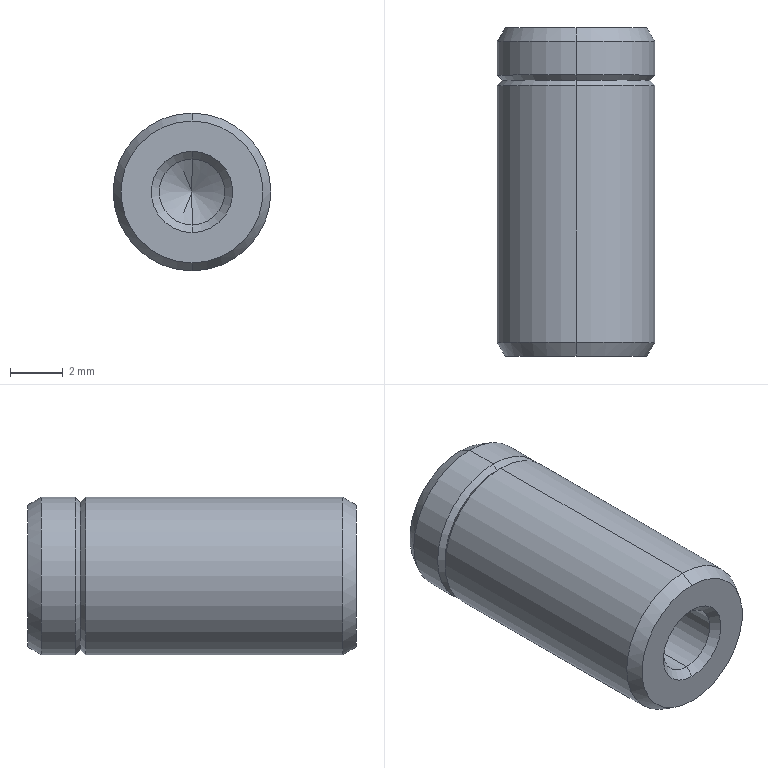Part | STEP file | MOP-12.5-1.step-2.STEP.STEP-60.STEP | 1 solid | 26 faces | box 6 x 12.5 x 6 mm | volume 302.452 mm3 | cone 16 | cylinder 8 | plane 2 | commonest cylinder face diameters 2.5 x4 6 x4
STEP:
#1=CARTESIAN_POINT('',(0.,10.3,3.));
#2=VERTEX_POINT('',#1);
#3=CARTESIAN_POINT('',(0.,10.3,-3.));
#4=VERTEX_POINT('',#3);
#5=CARTESIAN_POINT('',(0.,10.3,0.));
#6=DIRECTION('',(0.,1.,0.));
#7=DIRECTION('',(0.,0.,-1.));
#8=AXIS2_PLACEMENT_3D('',#5,#6,#7);
#9=CIRCLE('',#8,3.);
#10=EDGE_CURVE('',#2,#4,#9,.T.);
#11=ORIENTED_EDGE('',*,*,#10,.F.);
#12=CARTESIAN_POINT('',(0.,0.5196,3.));
#13=VERTEX_POINT('',#12);
#14=CARTESIAN_POINT('',(0.,12.5,3.));
#15=DIRECTION('',(0.,-1.,0.));
#16=VECTOR('',#15,1000.);
#17=LINE('',#14,#16);
#18=EDGE_CURVE('',#2,#13,#17,.T.);
#19=ORIENTED_EDGE('',*,*,#18,.T.);
#20=CARTESIAN_POINT('',(0.,0.5196,-3.));
#21=VERTEX_POINT('',#20);
#22=CARTESIAN_POINT('',(0.,0.5196,0.));
#23=DIRECTION('',(0.,1.,0.));
#24=DIRECTION('',(0.,0.,1.));
#25=AXIS2_PLACEMENT_3D('',#22,#23,#24);
#26=CIRCLE('',#25,3.);
#27=EDGE_CURVE('',#13,#21,#26,.T.);
#28=ORIENTED_EDGE('',*,*,#27,.T.);
#29=CARTESIAN_POINT('',(0.,12.5,-3.));
#30=DIRECTION('',(0.,-1.,0.));
#31=VECTOR('',#30,1000.);
#32=LINE('',#29,#31);
#33=EDGE_CURVE('',#4,#21,#32,.T.);
#34=ORIENTED_EDGE('',*,*,#33,.F.);
#35=EDGE_LOOP('',(#11,#19,#28,#34));
#36=FACE_OUTER_BOUND('',#35,.T.);
#37=CARTESIAN_POINT('',(0.,12.5,0.));
#38=DIRECTION('',(0.,-1.,0.));
#39=DIRECTION('',(0.,0.,-1.));
#40=AXIS2_PLACEMENT_3D('',#37,#38,#39);
#41=CYLINDRICAL_SURFACE('',#40,3.);
#42=ADVANCED_FACE('',(#36),#41,.T.);
#43=CARTESIAN_POINT('',(0.,0.,-2.7));
#44=VERTEX_POINT('',#43);
#45=CARTESIAN_POINT('',(0.,0.,2.7));
#46=VERTEX_POINT('',#45);
#47=CARTESIAN_POINT('',(0.,0.,0.));
#48=DIRECTION('',(0.,-1.,0.));
#49=DIRECTION('',(0.,0.,1.));
#50=AXIS2_PLACEMENT_3D('',#47,#48,#49);
#51=CIRCLE('',#50,2.7);
#52=EDGE_CURVE('',#44,#46,#51,.T.);
#53=ORIENTED_EDGE('',*,*,#52,.F.);
#54=CARTESIAN_POINT('',(0.,0.5196,-3.));
#55=DIRECTION('',(0.,0.866,-0.5));
#56=VECTOR('',#55,1000.);
#57=LINE('',#54,#56);
#58=EDGE_CURVE('',#44,#21,#57,.T.);
#59=ORIENTED_EDGE('',*,*,#58,.T.);
#60=ORIENTED_EDGE('',*,*,#27,.F.);
#61=CARTESIAN_POINT('',(0.,0.5196,3.));
#62=DIRECTION('',(0.,0.866,0.5));
#63=VECTOR('',#62,1000.);
#64=LINE('',#61,#63);
#65=EDGE_CURVE('',#46,#13,#64,.T.);
#66=ORIENTED_EDGE('',*,*,#65,.F.);
#67=EDGE_LOOP('',(#53,#59,#60,#66));
#68=FACE_OUTER_BOUND('',#67,.T.);
#69=CARTESIAN_POINT('',(0.,0.5196,0.));
#70=DIRECTION('',(0.,1.,0.));
#71=DIRECTION('',(0.,0.,1.));
#72=AXIS2_PLACEMENT_3D('',#69,#70,#71);
#73=CONICAL_SURFACE('',#72,3.,0.5236);
#74=ADVANCED_FACE('',(#68),#73,.T.);
#75=CARTESIAN_POINT('',(0.,0.3,1.25));
#76=VERTEX_POINT('',#75);
#77=CARTESIAN_POINT('',(0.,0.3,-1.25));
#78=VERTEX_POINT('',#77);
#79=CARTESIAN_POINT('',(0.,0.3,0.));
#80=DIRECTION('',(0.,-1.,0.));
#81=DIRECTION('',(0.,0.,1.));
#82=AXIS2_PLACEMENT_3D('',#79,#80,#81);
#83=CIRCLE('',#82,1.25);
#84=EDGE_CURVE('',#76,#78,#83,.T.);
#85=ORIENTED_EDGE('',*,*,#84,.F.);
#86=CARTESIAN_POINT('',(0.,0.,1.55));
#87=VERTEX_POINT('',#86);
#88=CARTESIAN_POINT('',(0.,0.3,1.25));
#89=DIRECTION('',(0.,-0.7071,0.7071));
#90=VECTOR('',#89,1000.);
#91=LINE('',#88,#90);
#92=EDGE_CURVE('',#76,#87,#91,.T.);
#93=ORIENTED_EDGE('',*,*,#92,.T.);
#94=CARTESIAN_POINT('',(0.,0.,-1.55));
#95=VERTEX_POINT('',#94);
#96=CARTESIAN_POINT('',(0.,0.,0.));
#97=DIRECTION('',(0.,1.,0.));
#98=DIRECTION('',(0.,0.,1.));
#99=AXIS2_PLACEMENT_3D('',#96,#97,#98);
#100=CIRCLE('',#99,1.55);
#101=EDGE_CURVE('',#95,#87,#100,.T.);
#102=ORIENTED_EDGE('',*,*,#101,.F.);
#103=CARTESIAN_POINT('',(0.,0.3,-1.25));
#104=DIRECTION('',(0.,-0.7071,-0.7071));
#105=VECTOR('',#104,1000.);
#106=LINE('',#103,#105);
#107=EDGE_CURVE('',#78,#95,#106,.T.);
#108=ORIENTED_EDGE('',*,*,#107,.F.);
#109=EDGE_LOOP('',(#85,#93,#102,#108));
#110=FACE_OUTER_BOUND('',#109,.T.);
#111=CARTESIAN_POINT('',(0.,0.3,0.));
#112=DIRECTION('',(0.,-1.,0.));
#113=DIRECTION('',(0.,0.,-1.));
#114=AXIS2_PLACEMENT_3D('',#111,#112,#113);
#115=CONICAL_SURFACE('',#114,1.25,0.7854);
#116=ADVANCED_FACE('',(#110),#115,.F.);
#117=CARTESIAN_POINT('',(0.,4.5,1.25));
#118=VERTEX_POINT('',#117);
#119=CARTESIAN_POINT('',(0.,4.5,-1.25));
#120=VERTEX_POINT('',#119);
#121=CARTESIAN_POINT('',(0.,4.5,0.));
#122=DIRECTION('',(0.,-1.,0.));
#123=DIRECTION('',(0.,0.,-1.));
#124=AXIS2_PLACEMENT_3D('',#121,#122,#123);
#125=CIRCLE('',#124,1.25);
#126=EDGE_CURVE('',#118,#120,#125,.T.);
#127=ORIENTED_EDGE('',*,*,#126,.F.);
#128=CARTESIAN_POINT('',(0.,0.,1.25));
#129=DIRECTION('',(0.,-1.,0.));
#130=VECTOR('',#129,1000.);
#131=LINE('',#128,#130);
#132=EDGE_CURVE('',#118,#76,#131,.T.);
#133=ORIENTED_EDGE('',*,*,#132,.T.);
#134=ORIENTED_EDGE('',*,*,#84,.T.);
#135=CARTESIAN_POINT('',(0.,0.,-1.25));
#136=DIRECTION('',(0.,-1.,0.));
#137=VECTOR('',#136,1000.);
#138=LINE('',#135,#137);
#139=EDGE_CURVE('',#120,#78,#138,.T.);
#140=ORIENTED_EDGE('',*,*,#139,.F.);
#141=EDGE_LOOP('',(#127,#133,#134,#140));
#142=FACE_OUTER_BOUND('',#141,.T.);
#143=CARTESIAN_POINT('',(0.,0.,0.));
#144=DIRECTION('',(0.,-1.,0.));
#145=DIRECTION('',(0.,0.,-1.));
#146=AXIS2_PLACEMENT_3D('',#143,#144,#145);
#147=CYLINDRICAL_SURFACE('',#146,1.25);
#148=ADVANCED_FACE('',(#142),#147,.F.);
#149=CARTESIAN_POINT('',(0.,5.251,0.));
#150=VERTEX_POINT('',#149);
#151=CARTESIAN_POINT('',(0.,4.5,-1.25));
#152=DIRECTION('',(0.,-0.515,-0.8572));
#153=VECTOR('',#152,1000.);
#154=LINE('',#151,#153);
#155=EDGE_CURVE('',#150,#120,#154,.T.);
#156=ORIENTED_EDGE('',*,*,#155,.F.);
#157=CARTESIAN_POINT('',(0.,4.5,1.25));
#158=DIRECTION('',(0.,-0.515,0.8572));
#159=VECTOR('',#158,1000.);
#160=LINE('',#157,#159);
#161=EDGE_CURVE('',#150,#118,#160,.T.);
#162=ORIENTED_EDGE('',*,*,#161,.T.);
#163=ORIENTED_EDGE('',*,*,#126,.T.);
#164=EDGE_LOOP('',(#156,#162,#163));
#165=FACE_OUTER_BOUND('',#164,.T.);
#166=CARTESIAN_POINT('',(0.,4.5,0.));
#167=DIRECTION('',(0.,-1.,0.));
#168=DIRECTION('',(0.,0.,-1.));
#169=AXIS2_PLACEMENT_3D('',#166,#167,#168);
#170=CONICAL_SURFACE('',#169,1.25,1.03);
#171=ADVANCED_FACE('',(#165),#170,.F.);
#172=CARTESIAN_POINT('',(0.,10.5,-2.8));
#173=VERTEX_POINT('',#172);
#174=CARTESIAN_POINT('',(0.,10.5,2.8));
#175=VERTEX_POINT('',#174);
#176=CARTESIAN_POINT('',(0.,10.5,0.));
#177=DIRECTION('',(0.,-1.,0.));
#178=DIRECTION('',(0.,0.,-1.));
#179=AXIS2_PLACEMENT_3D('',#176,#177,#178);
#180=CIRCLE('',#179,2.8);
#181=EDGE_CURVE('',#173,#175,#180,.T.);
#182=ORIENTED_EDGE('',*,*,#181,.T.);
#183=CARTESIAN_POINT('',(0.,-204.056,217.356));
#184=DIRECTION('',(0.,-0.7071,0.7071));
#185=VECTOR('',#184,1000.);
#186=LINE('',#183,#185);
#187=EDGE_CURVE('',#175,#2,#186,.T.);
#188=ORIENTED_EDGE('',*,*,#187,.T.);
#189=ORIENTED_EDGE('',*,*,#10,.T.);
#190=CARTESIAN_POINT('',(0.,-204.056,-217.356));
#191=DIRECTION('',(0.,-0.7071,-0.7071));
#192=VECTOR('',#191,1000.);
#193=LINE('',#190,#192);
#194=EDGE_CURVE('',#173,#4,#193,.T.);
#195=ORIENTED_EDGE('',*,*,#194,.F.);
#196=EDGE_LOOP('',(#182,#188,#189,#195));
#197=FACE_OUTER_BOUND('',#196,.T.);
#198=CARTESIAN_POINT('',(0.,-204.056,0.));
#199=DIRECTION('',(0.,-1.,0.));
#200=DIRECTION('',(0.,0.,-1.));
#201=AXIS2_PLACEMENT_3D('',#198,#199,#200);
#202=CONICAL_SURFACE('',#201,217.356,0.7854);
#203=ADVANCED_FACE('',(#197),#202,.T.);
#204=ORIENTED_EDGE('',*,*,#181,.F.);
#205=CARTESIAN_POINT('',(0.,10.7,-3.));
#206=VERTEX_POINT('',#205);
#207=CARTESIAN_POINT('',(0.,10.5,-2.8));
#208=DIRECTION('',(0.,0.7071,-0.7071));
#209=VECTOR('',#208,1000.);
#210=LINE('',#207,#209);
#211=EDGE_CURVE('',#173,#206,#210,.T.);
#212=ORIENTED_EDGE('',*,*,#211,.T.);
#213=CARTESIAN_POINT('',(0.,10.7,3.));
#214=VERTEX_POINT('',#213);
#215=CARTESIAN_POINT('',(0.,10.7,0.));
#216=DIRECTION('',(0.,-1.,0.));
#217=DIRECTION('',(0.,0.,1.));
#218=AXIS2_PLACEMENT_3D('',#215,#216,#217);
#219=CIRCLE('',#218,3.);
#220=EDGE_CURVE('',#206,#214,#219,.T.);
#221=ORIENTED_EDGE('',*,*,#220,.T.);
#222=CARTESIAN_POINT('',(0.,10.5,2.8));
#223=DIRECTION('',(0.,0.7071,0.7071));
#224=VECTOR('',#223,1000.);
#225=LINE('',#222,#224);
#226=EDGE_CURVE('',#175,#214,#225,.T.);
#227=ORIENTED_EDGE('',*,*,#226,.F.);
#228=EDGE_LOOP('',(#204,#212,#221,#227));
#229=FACE_OUTER_BOUND('',#228,.T.);
#230=CARTESIAN_POINT('',(0.,10.5,0.));
#231=DIRECTION('',(0.,1.,0.));
#232=DIRECTION('',(0.,0.,1.));
#233=AXIS2_PLACEMENT_3D('',#230,#231,#232);
#234=CONICAL_SURFACE('',#233,2.8,0.7854);
#235=ADVANCED_FACE('',(#229),#234,.T.);
#236=CARTESIAN_POINT('',(0.,12.2,-1.25));
#237=VERTEX_POINT('',#236);
#238=CARTESIAN_POINT('',(0.,12.2,1.25));
#239=VERTEX_POINT('',#238);
#240=CARTESIAN_POINT('',(0.,12.2,0.));
#241=DIRECTION('',(0.,1.,0.));
#242=DIRECTION('',(0.,0.,1.));
#243=AXIS2_PLACEMENT_3D('',#240,#241,#242);
#244=CIRCLE('',#243,1.25);
#245=EDGE_CURVE('',#237,#239,#244,.T.);
#246=ORIENTED_EDGE('',*,*,#245,.F.);
#247=CARTESIAN_POINT('',(0.,12.5,-1.55));
#248=VERTEX_POINT('',#247);
#249=CARTESIAN_POINT('',(0.,12.2,-1.25));
#250=DIRECTION('',(0.,0.7071,-0.7071));
#251=VECTOR('',#250,1000.);
#252=LINE('',#249,#251);
#253=EDGE_CURVE('',#237,#248,#252,.T.);
#254=ORIENTED_EDGE('',*,*,#253,.T.);
#255=CARTESIAN_POINT('',(0.,12.5,1.55));
#256=VERTEX_POINT('',#255);
#257=CARTESIAN_POINT('',(0.,12.5,0.));
#258=DIRECTION('',(0.,-1.,0.));
#259=DIRECTION('',(0.,0.,1.));
#260=AXIS2_PLACEMENT_3D('',#257,#258,#259);
#261=CIRCLE('',#260,1.55);
#262=EDGE_CURVE('',#256,#248,#261,.T.);
#263=ORIENTED_EDGE('',*,*,#262,.F.);
#264=CARTESIAN_POINT('',(0.,12.2,1.25));
#265=DIRECTION('',(0.,0.7071,0.7071));
#266=VECTOR('',#265,1000.);
#267=LINE('',#264,#266);
#268=EDGE_CURVE('',#239,#256,#267,.T.);
#269=ORIENTED_EDGE('',*,*,#268,.F.);
#270=EDGE_LOOP('',(#246,#254,#263,#269));
#271=FACE_OUTER_BOUND('',#270,.T.);
#272=CARTESIAN_POINT('',(0.,12.2,0.));
#273=DIRECTION('',(0.,1.,0.));
#274=DIRECTION('',(0.,0.,1.));
#275=AXIS2_PLACEMENT_3D('',#272,#273,#274);
#276=CONICAL_SURFACE('',#275,1.25,0.7854);
#277=ADVANCED_FACE('',(#271),#276,.F.);
#278=CARTESIAN_POINT('',(0.,12.5,2.7));
#279=VERTEX_POINT('',#278);
#280=CARTESIAN_POINT('',(0.,12.5,-2.7));
#281=VERTEX_POINT('',#280);
#282=CARTESIAN_POINT('',(0.,12.5,0.));
#283=DIRECTION('',(0.,1.,0.));
#284=DIRECTION('',(0.,0.,1.));
#285=AXIS2_PLACEMENT_3D('',#282,#283,#284);
#286=CIRCLE('',#285,2.7);
#287=EDGE_CURVE('',#279,#281,#286,.T.);
#288=ORIENTED_EDGE('',*,*,#287,.F.);
#289=CARTESIAN_POINT('',(0.,11.98,3.));
#290=VERTEX_POINT('',#289);
#291=CARTESIAN_POINT('',(0.,12.5,2.7));
#292=DIRECTION('',(0.,-0.866,0.5));
#293=VECTOR('',#292,1000.);
#294=LINE('',#291,#293);
#295=EDGE_CURVE('',#279,#290,#294,.T.);
#296=ORIENTED_EDGE('',*,*,#295,.T.);
#297=CARTESIAN_POINT('',(0.,11.98,-3.));
#298=VERTEX_POINT('',#297);
#299=CARTESIAN_POINT('',(0.,11.98,0.));
#300=DIRECTION('',(0.,-1.,0.));
#301=DIRECTION('',(0.,0.,1.));
#302=AXIS2_PLACEMENT_3D('',#299,#300,#301);
#303=CIRCLE('',#302,3.);
#304=EDGE_CURVE('',#298,#290,#303,.T.);
#305=ORIENTED_EDGE('',*,*,#304,.F.);
#306=CARTESIAN_POINT('',(0.,12.5,-2.7));
#307=DIRECTION('',(0.,-0.866,-0.5));
#308=VECTOR('',#307,1000.);
#309=LINE('',#306,#308);
#310=EDGE_CURVE('',#281,#298,#309,.T.);
#311=ORIENTED_EDGE('',*,*,#310,.F.);
#312=EDGE_LOOP('',(#288,#296,#305,#311));
#313=FACE_OUTER_BOUND('',#312,.T.);
#314=CARTESIAN_POINT('',(0.,12.5,0.));
#315=DIRECTION('',(0.,-1.,0.));
#316=DIRECTION('',(0.,0.,-1.));
#317=AXIS2_PLACEMENT_3D('',#314,#315,#316);
#318=CONICAL_SURFACE('',#317,2.7,0.5236);
#319=ADVANCED_FACE('',(#313),#318,.T.);
#320=CARTESIAN_POINT('',(0.,8.,-1.25));
#321=VERTEX_POINT('',#320);
#322=CARTESIAN_POINT('',(0.,8.,1.25));
#323=VERTEX_POINT('',#322);
#324=CARTESIAN_POINT('',(0.,8.,0.));
#325=DIRECTION('',(0.,1.,0.));
#326=DIRECTION('',(0.,0.,1.));
#327=AXIS2_PLACEMENT_3D('',#324,#325,#326);
#328=CIRCLE('',#327,1.25);
#329=EDGE_CURVE('',#321,#323,#328,.T.);
#330=ORIENTED_EDGE('',*,*,#329,.F.);
#331=CARTESIAN_POINT('',(0.,12.5,-1.25));
#332=DIRECTION('',(0.,1.,0.));
#333=VECTOR('',#332,1000.);
#334=LINE('',#331,#333);
#335=EDGE_CURVE('',#321,#237,#334,.T.);
#336=ORIENTED_EDGE('',*,*,#335,.T.);
#337=ORIENTED_EDGE('',*,*,#245,.T.);
#338=CARTESIAN_POINT('',(0.,12.5,1.25));
#339=DIRECTION('',(0.,1.,0.));
#340=VECTOR('',#339,1000.);
#341=LINE('',#338,#340);
#342=EDGE_CURVE('',#323,#239,#341,.T.);
#343=ORIENTED_EDGE('',*,*,#342,.F.);
#344=EDGE_LOOP('',(#330,#336,#337,#343));
#345=FACE_OUTER_BOUND('',#344,.T.);
#346=CARTESIAN_POINT('',(0.,12.5,0.));
#347=DIRECTION('',(0.,1.,0.));
#348=DIRECTION('',(0.,0.,1.));
#349=AXIS2_PLACEMENT_3D('',#346,#347,#348);
#350=CYLINDRICAL_SURFACE('',#349,1.25);
#351=ADVANCED_FACE('',(#345),#350,.F.);
#352=CARTESIAN_POINT('',(0.,7.249,0.));
#353=VERTEX_POINT('',#352);
#354=CARTESIAN_POINT('',(0.,8.,1.25));
#355=DIRECTION('',(0.,0.515,0.8572));
#356=VECTOR('',#355,1000.);
#357=LINE('',#354,#356);
#358=EDGE_CURVE('',#353,#323,#357,.T.);
#359=ORIENTED_EDGE('',*,*,#358,.F.);
#360=CARTESIAN_POINT('',(0.,8.,-1.25));
#361=DIRECTION('',(0.,0.515,-0.8572));
#362=VECTOR('',#361,1000.);
#363=LINE('',#360,#362);
#364=EDGE_CURVE('',#353,#321,#363,.T.);
#365=ORIENTED_EDGE('',*,*,#364,.T.);
#366=ORIENTED_EDGE('',*,*,#329,.T.);
#367=EDGE_LOOP('',(#359,#365,#366));
#368=FACE_OUTER_BOUND('',#367,.T.);
#369=CARTESIAN_POINT('',(0.,8.,0.));
#370=DIRECTION('',(0.,1.,0.));
#371=DIRECTION('',(0.,0.,1.));
#372=AXIS2_PLACEMENT_3D('',#369,#370,#371);
#373=CONICAL_SURFACE('',#372,1.25,1.03);
#374=ADVANCED_FACE('',(#368),#373,.F.);
#375=ORIENTED_EDGE('',*,*,#304,.T.);
#376=CARTESIAN_POINT('',(0.,12.5,3.));
#377=DIRECTION('',(0.,-1.,0.));
#378=VECTOR('',#377,1000.);
#379=LINE('',#376,#378);
#380=EDGE_CURVE('',#290,#214,#379,.T.);
#381=ORIENTED_EDGE('',*,*,#380,.T.);
#382=ORIENTED_EDGE('',*,*,#220,.F.);
#383=CARTESIAN_POINT('',(0.,12.5,-3.));
#384=DIRECTION('',(0.,-1.,0.));
#385=VECTOR('',#384,1000.);
#386=LINE('',#383,#385);
#387=EDGE_CURVE('',#298,#206,#386,.T.);
#388=ORIENTED_EDGE('',*,*,#387,.F.);
#389=EDGE_LOOP('',(#375,#381,#382,#388));
#390=FACE_OUTER_BOUND('',#389,.T.);
#391=CARTESIAN_POINT('',(0.,12.5,0.));
#392=DIRECTION('',(0.,-1.,0.));
#393=DIRECTION('',(0.,0.,-1.));
#394=AXIS2_PLACEMENT_3D('',#391,#392,#393);
#395=CYLINDRICAL_SURFACE('',#394,3.);
#396=ADVANCED_FACE('',(#390),#395,.T.);
#397=ORIENTED_EDGE('',*,*,#380,.F.);
#398=CARTESIAN_POINT('',(0.,11.98,0.));
#399=DIRECTION('',(0.,-1.,0.));
#400=DIRECTION('',(0.,0.,1.));
#401=AXIS2_PLACEMENT_3D('',#398,#399,#400);
#402=CIRCLE('',#401,3.);
#403=EDGE_CURVE('',#290,#298,#402,.T.);
#404=ORIENTED_EDGE('',*,*,#403,.T.);
#405=ORIENTED_EDGE('',*,*,#387,.T.);
#406=CARTESIAN_POINT('',(0.,10.7,0.));
#407=DIRECTION('',(0.,-1.,0.));
#408=DIRECTION('',(0.,0.,1.));
#409=AXIS2_PLACEMENT_3D('',#406,#407,#408);
#410=CIRCLE('',#409,3.);
#411=EDGE_CURVE('',#214,#206,#410,.T.);
#412=ORIENTED_EDGE('',*,*,#411,.F.);
#413=EDGE_LOOP('',(#397,#404,#405,#412));
#414=FACE_OUTER_BOUND('',#413,.T.);
#415=CARTESIAN_POINT('',(0.,12.5,0.));
#416=DIRECTION('',(0.,-1.,0.));
#417=DIRECTION('',(0.,0.,-1.));
#418=AXIS2_PLACEMENT_3D('',#415,#416,#417);
#419=CYLINDRICAL_SURFACE('',#418,3.);
#420=ADVANCED_FACE('',(#414),#419,.T.);
#421=ORIENTED_EDGE('',*,*,#262,.T.);
#422=CARTESIAN_POINT('',(0.,12.5,0.));
#423=DIRECTION('',(0.,-1.,0.));
#424=DIRECTION('',(0.,0.,1.));
#425=AXIS2_PLACEMENT_3D('',#422,#423,#424);
#426=CIRCLE('',#425,1.55);
#427=EDGE_CURVE('',#248,#256,#426,.T.);
#428=ORIENTED_EDGE('',*,*,#427,.T.);
#429=EDGE_LOOP('',(#421,#428));
#430=FACE_BOUND('',#429,.T.);
#431=CARTESIAN_POINT('',(0.,12.5,0.));
#432=DIRECTION('',(0.,1.,0.));
#433=DIRECTION('',(0.,0.,1.));
#434=AXIS2_PLACEMENT_3D('',#431,#432,#433);
#435=CIRCLE('',#434,2.7);
#436=EDGE_CURVE('',#281,#279,#435,.T.);
#437=ORIENTED_EDGE('',*,*,#436,.T.);
#438=ORIENTED_EDGE('',*,*,#287,.T.);
#439=EDGE_LOOP('',(#437,#438));
#440=FACE_OUTER_BOUND('',#439,.T.);
#441=CARTESIAN_POINT('',(0.,12.5,0.));
#442=DIRECTION('',(0.,1.,0.));
#443=DIRECTION('',(1.,0.,0.));
#444=AXIS2_PLACEMENT_3D('',#441,#442,#443);
#445=PLANE('',#444);
#446=ADVANCED_FACE('',(#430,#440),#445,.T.);
#447=ORIENTED_EDGE('',*,*,#364,.F.);
#448=ORIENTED_EDGE('',*,*,#358,.T.);
#449=CARTESIAN_POINT('',(0.,8.,0.));
#450=DIRECTION('',(0.,1.,0.));
#451=DIRECTION('',(0.,0.,1.));
#452=AXIS2_PLACEMENT_3D('',#449,#450,#451);
#453=CIRCLE('',#452,1.25);
#454=EDGE_CURVE('',#323,#321,#453,.T.);
#455=ORIENTED_EDGE('',*,*,#454,.T.);
#456=EDGE_LOOP('',(#447,#448,#455));
#457=FACE_OUTER_BOUND('',#456,.T.);
#458=CARTESIAN_POINT('',(0.,8.,0.));
#459=DIRECTION('',(0.,1.,0.));
#460=DIRECTION('',(0.,0.,1.));
#461=AXIS2_PLACEMENT_3D('',#458,#459,#460);
#462=CONICAL_SURFACE('',#461,1.25,1.03);
#463=ADVANCED_FACE('',(#457),#462,.F.);
#464=ORIENTED_EDGE('',*,*,#335,.F.);
#465=ORIENTED_EDGE('',*,*,#454,.F.);
#466=ORIENTED_EDGE('',*,*,#342,.T.);
#467=CARTESIAN_POINT('',(0.,12.2,0.));
#468=DIRECTION('',(0.,1.,0.));
#469=DIRECTION('',(0.,0.,1.));
#470=AXIS2_PLACEMENT_3D('',#467,#468,#469);
#471=CIRCLE('',#470,1.25);
#472=EDGE_CURVE('',#239,#237,#471,.T.);
#473=ORIENTED_EDGE('',*,*,#472,.T.);
#474=EDGE_LOOP('',(#464,#465,#466,#473));
#475=FACE_OUTER_BOUND('',#474,.T.);
#476=CARTESIAN_POINT('',(0.,12.5,0.));
#477=DIRECTION('',(0.,1.,0.));
#478=DIRECTION('',(0.,0.,1.));
#479=AXIS2_PLACEMENT_3D('',#476,#477,#478);
#480=CYLINDRICAL_SURFACE('',#479,1.25);
#481=ADVANCED_FACE('',(#475),#480,.F.);
#482=ORIENTED_EDGE('',*,*,#295,.F.);
#483=ORIENTED_EDGE('',*,*,#436,.F.);
#484=ORIENTED_EDGE('',*,*,#310,.T.);
#485=ORIENTED_EDGE('',*,*,#403,.F.);
#486=EDGE_LOOP('',(#482,#483,#484,#485));
#487=FACE_OUTER_BOUND('',#486,.T.);
#488=CARTESIAN_POINT('',(0.,12.5,0.));
#489=DIRECTION('',(0.,-1.,0.));
#490=DIRECTION('',(0.,0.,-1.));
#491=AXIS2_PLACEMENT_3D('',#488,#489,#490);
#492=CONICAL_SURFACE('',#491,2.7,0.5236);
#493=ADVANCED_FACE('',(#487),#492,.T.);
#494=ORIENTED_EDGE('',*,*,#253,.F.);
#495=ORIENTED_EDGE('',*,*,#472,.F.);
#496=ORIENTED_EDGE('',*,*,#268,.T.);
#497=ORIENTED_EDGE('',*,*,#427,.F.);
#498=EDGE_LOOP('',(#494,#495,#496,#497));
#499=FACE_OUTER_BOUND('',#498,.T.);
#500=CARTESIAN_POINT('',(0.,12.2,0.));
#501=DIRECTION('',(0.,1.,0.));
#502=DIRECTION('',(0.,0.,1.));
#503=AXIS2_PLACEMENT_3D('',#500,#501,#502);
#504=CONICAL_SURFACE('',#503,1.25,0.7854);
#505=ADVANCED_FACE('',(#499),#504,.F.);
#506=ORIENTED_EDGE('',*,*,#211,.F.);
#507=CARTESIAN_POINT('',(0.,10.5,0.));
#508=DIRECTION('',(0.,-1.,0.));
#509=DIRECTION('',(0.,0.,-1.));
#510=AXIS2_PLACEMENT_3D('',#507,#508,#509);
#511=CIRCLE('',#510,2.8);
#512=EDGE_CURVE('',#175,#173,#511,.T.);
#513=ORIENTED_EDGE('',*,*,#512,.F.);
#514=ORIENTED_EDGE('',*,*,#226,.T.);
#515=ORIENTED_EDGE('',*,*,#411,.T.);
#516=EDGE_LOOP('',(#506,#513,#514,#515));
#517=FACE_OUTER_BOUND('',#516,.T.);
#518=CARTESIAN_POINT('',(0.,10.5,0.));
#519=DIRECTION('',(0.,1.,0.));
#520=DIRECTION('',(0.,0.,1.));
#521=AXIS2_PLACEMENT_3D('',#518,#519,#520);
#522=CONICAL_SURFACE('',#521,2.8,0.7854);
#523=ADVANCED_FACE('',(#517),#522,.T.);
#524=ORIENTED_EDGE('',*,*,#187,.F.);
#525=ORIENTED_EDGE('',*,*,#512,.T.);
#526=ORIENTED_EDGE('',*,*,#194,.T.);
#527=CARTESIAN_POINT('',(0.,10.3,0.));
#528=DIRECTION('',(0.,1.,0.));
#529=DIRECTION('',(0.,0.,-1.));
#530=AXIS2_PLACEMENT_3D('',#527,#528,#529);
#531=CIRCLE('',#530,3.);
#532=EDGE_CURVE('',#4,#2,#531,.T.);
#533=ORIENTED_EDGE('',*,*,#532,.T.);
#534=EDGE_LOOP('',(#524,#525,#526,#533));
#535=FACE_OUTER_BOUND('',#534,.T.);
#536=CARTESIAN_POINT('',(0.,-204.056,0.));
#537=DIRECTION('',(0.,-1.,0.));
#538=DIRECTION('',(0.,0.,-1.));
#539=AXIS2_PLACEMENT_3D('',#536,#537,#538);
#540=CONICAL_SURFACE('',#539,217.356,0.7854);
#541=ADVANCED_FACE('',(#535),#540,.T.);
#542=ORIENTED_EDGE('',*,*,#161,.F.);
#543=ORIENTED_EDGE('',*,*,#155,.T.);
#544=CARTESIAN_POINT('',(0.,4.5,0.));
#545=DIRECTION('',(0.,-1.,0.));
#546=DIRECTION('',(0.,0.,-1.));
#547=AXIS2_PLACEMENT_3D('',#544,#545,#546);
#548=CIRCLE('',#547,1.25);
#549=EDGE_CURVE('',#120,#118,#548,.T.);
#550=ORIENTED_EDGE('',*,*,#549,.T.);
#551=EDGE_LOOP('',(#542,#543,#550));
#552=FACE_OUTER_BOUND('',#551,.T.);
#553=CARTESIAN_POINT('',(0.,4.5,0.));
#554=DIRECTION('',(0.,-1.,0.));
#555=DIRECTION('',(0.,0.,-1.));
#556=AXIS2_PLACEMENT_3D('',#553,#554,#555);
#557=CONICAL_SURFACE('',#556,1.25,1.03);
#558=ADVANCED_FACE('',(#552),#557,.F.);
#559=ORIENTED_EDGE('',*,*,#132,.F.);
#560=ORIENTED_EDGE('',*,*,#549,.F.);
#561=ORIENTED_EDGE('',*,*,#139,.T.);
#562=CARTESIAN_POINT('',(0.,0.3,0.));
#563=DIRECTION('',(0.,-1.,0.));
#564=DIRECTION('',(0.,0.,1.));
#565=AXIS2_PLACEMENT_3D('',#562,#563,#564);
#566=CIRCLE('',#565,1.25);
#567=EDGE_CURVE('',#78,#76,#566,.T.);
#568=ORIENTED_EDGE('',*,*,#567,.T.);
#569=EDGE_LOOP('',(#559,#560,#561,#568));
#570=FACE_OUTER_BOUND('',#569,.T.);
#571=CARTESIAN_POINT('',(0.,0.,0.));
#572=DIRECTION('',(0.,-1.,0.));
#573=DIRECTION('',(0.,0.,-1.));
#574=AXIS2_PLACEMENT_3D('',#571,#572,#573);
#575=CYLINDRICAL_SURFACE('',#574,1.25);
#576=ADVANCED_FACE('',(#570),#575,.F.);
#577=ORIENTED_EDGE('',*,*,#92,.F.);
#578=ORIENTED_EDGE('',*,*,#567,.F.);
#579=ORIENTED_EDGE('',*,*,#107,.T.);
#580=CARTESIAN_POINT('',(0.,0.,0.));
#581=DIRECTION('',(0.,1.,0.));
#582=DIRECTION('',(0.,0.,1.));
#583=AXIS2_PLACEMENT_3D('',#580,#581,#582);
#584=CIRCLE('',#583,1.55);
#585=EDGE_CURVE('',#87,#95,#584,.T.);
#586=ORIENTED_EDGE('',*,*,#585,.F.);
#587=EDGE_LOOP('',(#577,#578,#579,#586));
#588=FACE_OUTER_BOUND('',#587,.T.);
#589=CARTESIAN_POINT('',(0.,0.3,0.));
#590=DIRECTION('',(0.,-1.,0.));
#591=DIRECTION('',(0.,0.,-1.));
#592=AXIS2_PLACEMENT_3D('',#589,#590,#591);
#593=CONICAL_SURFACE('',#592,1.25,0.7854);
#594=ADVANCED_FACE('',(#588),#593,.F.);
#595=ORIENTED_EDGE('',*,*,#101,.T.);
#596=ORIENTED_EDGE('',*,*,#585,.T.);
#597=EDGE_LOOP('',(#595,#596));
#598=FACE_BOUND('',#597,.T.);
#599=CARTESIAN_POINT('',(0.,0.,0.));
#600=DIRECTION('',(0.,-1.,0.));
#601=DIRECTION('',(0.,0.,1.));
#602=AXIS2_PLACEMENT_3D('',#599,#600,#601);
#603=CIRCLE('',#602,2.7);
#604=EDGE_CURVE('',#46,#44,#603,.T.);
#605=ORIENTED_EDGE('',*,*,#604,.T.);
#606=ORIENTED_EDGE('',*,*,#52,.T.);
#607=EDGE_LOOP('',(#605,#606));
#608=FACE_OUTER_BOUND('',#607,.T.);
#609=CARTESIAN_POINT('',(0.,0.,0.));
#610=DIRECTION('',(0.,1.,0.));
#611=DIRECTION('',(1.,0.,0.));
#612=AXIS2_PLACEMENT_3D('',#609,#610,#611);
#613=PLANE('',#612);
#614=ADVANCED_FACE('',(#598,#608),#613,.F.);
#615=ORIENTED_EDGE('',*,*,#58,.F.);
#616=ORIENTED_EDGE('',*,*,#604,.F.);
#617=ORIENTED_EDGE('',*,*,#65,.T.);
#618=CARTESIAN_POINT('',(0.,0.5196,0.));
#619=DIRECTION('',(0.,1.,0.));
#620=DIRECTION('',(0.,0.,1.));
#621=AXIS2_PLACEMENT_3D('',#618,#619,#620);
#622=CIRCLE('',#621,3.);
#623=EDGE_CURVE('',#21,#13,#622,.T.);
#624=ORIENTED_EDGE('',*,*,#623,.F.);
#625=EDGE_LOOP('',(#615,#616,#617,#624));
#626=FACE_OUTER_BOUND('',#625,.T.);
#627=CARTESIAN_POINT('',(0.,0.5196,0.));
#628=DIRECTION('',(0.,1.,0.));
#629=DIRECTION('',(0.,0.,1.));
#630=AXIS2_PLACEMENT_3D('',#627,#628,#629);
#631=CONICAL_SURFACE('',#630,3.,0.5236);
#632=ADVANCED_FACE('',(#626),#631,.T.);
#633=ORIENTED_EDGE('',*,*,#18,.F.);
#634=ORIENTED_EDGE('',*,*,#532,.F.);
#635=ORIENTED_EDGE('',*,*,#33,.T.);
#636=ORIENTED_EDGE('',*,*,#623,.T.);
#637=EDGE_LOOP('',(#633,#634,#635,#636));
#638=FACE_OUTER_BOUND('',#637,.T.);
#639=CARTESIAN_POINT('',(0.,12.5,0.));
#640=DIRECTION('',(0.,-1.,0.));
#641=DIRECTION('',(0.,0.,-1.));
#642=AXIS2_PLACEMENT_3D('',#639,#640,#641);
#643=CYLINDRICAL_SURFACE('',#642,3.);
#644=ADVANCED_FACE('',(#638),#643,.T.);
#645=CLOSED_SHELL('',(#42,#74,#116,#148,#171,#203,#235,#277,#319,#351,#374,#396,#420,#446,#463,#481,#493,#505,#523,#541,#558,#576,#594,#614,#632,#644));
#646=MANIFOLD_SOLID_BREP('',#645);
#647=CARTESIAN_POINT('',(0.,0.,0.));
#648=DIRECTION('',(0.,0.,1.));
#649=DIRECTION('',(1.,0.,0.));
#650=AXIS2_PLACEMENT_3D('',#647,#648,#649);
#651=(LENGTH_UNIT()NAMED_UNIT(*)SI_UNIT(.MILLI.,.METRE.));
#652=UNCERTAINTY_MEASURE_WITH_UNIT(LENGTH_MEASURE(0.00001),#651,'','');
#653=(NAMED_UNIT(*)PLANE_ANGLE_UNIT()SI_UNIT($,.RADIAN.));
#654=(NAMED_UNIT(*)SI_UNIT($,.STERADIAN.)SOLID_ANGLE_UNIT());
#655=(GEOMETRIC_REPRESENTATION_CONTEXT(3)GLOBAL_UNCERTAINTY_ASSIGNED_CONTEXT((#652))GLOBAL_UNIT_ASSIGNED_CONTEXT((#651,#653,#654))REPRESENTATION_CONTEXT('',''));
#656=ADVANCED_BREP_SHAPE_REPRESENTATION('',(#646,#650),#655);